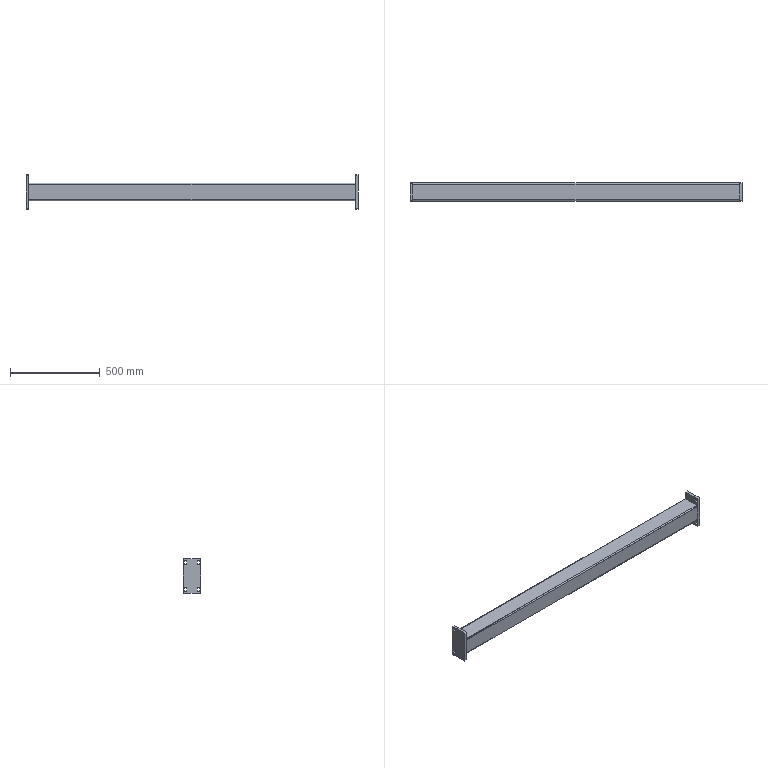Part | SolidWorks | features HoleWzd 1, ICE 1, MirrorSolid 1, WeldMemberFeat 1, WeldmentFeature 1 | 3 solids | 78 faces | box 1845 x 100 x 190 mm | volume 2736119 mm3 | plane 46 | cylinder 32 | commonest cylinder face diameters 13.5 x24 6.4 x4 12.8 x4